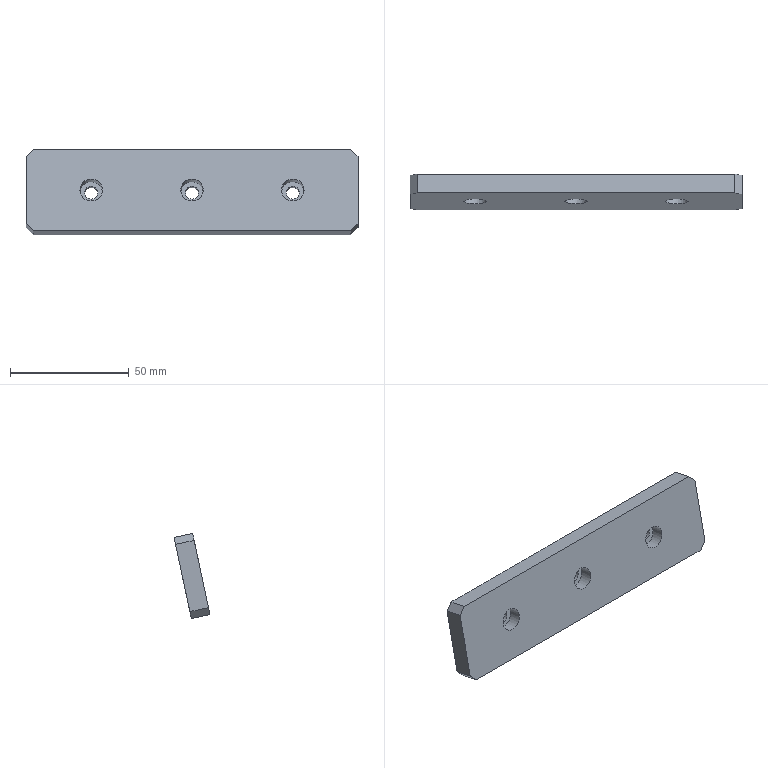Part | STEP file | P011002S004-005 | 1 solid | 19 faces | box 140 x 15.102 x 35.898 mm | volume 37708 mm3 | plane 13 | cylinder 6 | commonest cylinder face diameters 5.5 x3 9.5 x3
STEP:
#1=CARTESIAN_POINT('',(0.,0.,0.));
#2=DIRECTION('',(0.,0.,1.));
#3=DIRECTION('',(1.,0.,0.));
#4=AXIS2_PLACEMENT_3D('',#1,#2,#3);
#5=CARTESIAN_POINT('',(-47.25,-255.791,41.161));
#6=VERTEX_POINT('',#5);
#7=CARTESIAN_POINT('',(-42.5,-255.791,41.161));
#8=DIRECTION('',(0.,0.9781,-0.2079));
#9=DIRECTION('',(-1.,0.,0.));
#10=AXIS2_PLACEMENT_3D('',#7,#8,#9);
#11=CIRCLE('',#10,4.75);
#12=CARTESIAN_POINT('',(-5.,-253.192,53.388));
#13=DIRECTION('',(0.,-0.9781,0.2079));
#14=DIRECTION('',(0.,-0.2079,-0.9781));
#15=AXIS2_PLACEMENT_3D('',#12,#13,#14);
#16=PLANE('',#15);
#17=CARTESIAN_POINT('',(12.5,-42.25));
#18=CARTESIAN_POINT('',(4.273,-42.25));
#19=CARTESIAN_POINT('',(8.386,-35.125));
#20=CARTESIAN_POINT('',(12.5,-28.));
#21=CARTESIAN_POINT('',(16.614,-35.125));
#22=CARTESIAN_POINT('',(20.727,-42.25));
#23=CARTESIAN_POINT('',(12.5,-42.25));
#24=(BOUNDED_CURVE()B_SPLINE_CURVE(2,(#17,#18,#19,#20,#21,#22,#23),.UNSPECIFIED.,.T.,.F.)B_SPLINE_CURVE_WITH_KNOTS((1,2,2,2,2,1),(-2.094,0.,2.094,4.189,6.283,8.378),.UNSPECIFIED.)CURVE()GEOMETRIC_REPRESENTATION_ITEM()RATIONAL_B_SPLINE_CURVE((1.,0.5,1.,0.5,1.,0.5,1.))REPRESENTATION_ITEM(''));
#25=(GEOMETRIC_REPRESENTATION_CONTEXT(2)PARAMETRIC_REPRESENTATION_CONTEXT()REPRESENTATION_CONTEXT('',''));
#26=DEFINITIONAL_REPRESENTATION('',(#24),#25);
#27=PCURVE('',#16,#26);
#28=CARTESIAN_POINT('',(-42.5,-211.774,31.805));
#29=DIRECTION('',(0.,-0.9781,0.2079));
#30=DIRECTION('',(0.,-0.2079,-0.9781));
#31=AXIS2_PLACEMENT_3D('',#28,#29,#30);
#32=CYLINDRICAL_SURFACE('',#31,4.75);
#33=CARTESIAN_POINT('',(10.996,45.));
#34=DIRECTION('',(-1.,0.));
#35=VECTOR('',#34,1.);
#36=LINE('',#33,#35);
#37=(GEOMETRIC_REPRESENTATION_CONTEXT(2)PARAMETRIC_REPRESENTATION_CONTEXT()REPRESENTATION_CONTEXT('',''));
#38=DEFINITIONAL_REPRESENTATION('',(#36),#37);
#39=PCURVE('',#32,#38);
#40=SURFACE_CURVE('',#11,(#27,#39),.PCURVE_S1.);
#41=EDGE_CURVE('',#6,#6,#40,.T.);
#42=ORIENTED_EDGE('',*,*,#41,.T.);
#43=EDGE_LOOP('',(#42));
#44=FACE_BOUND('',#43,.T.);
#45=CARTESIAN_POINT('',(37.75,-255.791,41.161));
#46=VERTEX_POINT('',#45);
#47=CARTESIAN_POINT('',(42.5,-255.791,41.161));
#48=DIRECTION('',(0.,0.9781,-0.2079));
#49=DIRECTION('',(-1.,0.,0.));
#50=AXIS2_PLACEMENT_3D('',#47,#48,#49);
#51=CIRCLE('',#50,4.75);
#52=CARTESIAN_POINT('',(12.5,42.75));
#53=CARTESIAN_POINT('',(4.273,42.75));
#54=CARTESIAN_POINT('',(8.386,49.875));
#55=CARTESIAN_POINT('',(12.5,57.));
#56=CARTESIAN_POINT('',(16.614,49.875));
#57=CARTESIAN_POINT('',(20.727,42.75));
#58=CARTESIAN_POINT('',(12.5,42.75));
#59=(BOUNDED_CURVE()B_SPLINE_CURVE(2,(#52,#53,#54,#55,#56,#57,#58),.UNSPECIFIED.,.T.,.F.)B_SPLINE_CURVE_WITH_KNOTS((1,2,2,2,2,1),(-2.094,0.,2.094,4.189,6.283,8.378),.UNSPECIFIED.)CURVE()GEOMETRIC_REPRESENTATION_ITEM()RATIONAL_B_SPLINE_CURVE((1.,0.5,1.,0.5,1.,0.5,1.))REPRESENTATION_ITEM(''));
#60=(GEOMETRIC_REPRESENTATION_CONTEXT(2)PARAMETRIC_REPRESENTATION_CONTEXT()REPRESENTATION_CONTEXT('',''));
#61=DEFINITIONAL_REPRESENTATION('',(#59),#60);
#62=PCURVE('',#16,#61);
#63=CARTESIAN_POINT('',(42.5,-211.774,31.805));
#64=DIRECTION('',(0.,-0.9781,0.2079));
#65=DIRECTION('',(0.,-0.2079,-0.9781));
#66=AXIS2_PLACEMENT_3D('',#63,#64,#65);
#67=CYLINDRICAL_SURFACE('',#66,4.75);
#68=CARTESIAN_POINT('',(10.996,45.));
#69=DIRECTION('',(-1.,0.));
#70=VECTOR('',#69,1.);
#71=LINE('',#68,#70);
#72=(GEOMETRIC_REPRESENTATION_CONTEXT(2)PARAMETRIC_REPRESENTATION_CONTEXT()REPRESENTATION_CONTEXT('',''));
#73=DEFINITIONAL_REPRESENTATION('',(#71),#72);
#74=PCURVE('',#67,#73);
#75=SURFACE_CURVE('',#51,(#62,#74),.PCURVE_S1.);
#76=EDGE_CURVE('',#46,#46,#75,.T.);
#77=ORIENTED_EDGE('',*,*,#76,.T.);
#78=EDGE_LOOP('',(#77));
#79=FACE_BOUND('',#78,.T.);
#80=CARTESIAN_POINT('',(-4.75,-255.791,41.161));
#81=VERTEX_POINT('',#80);
#82=CARTESIAN_POINT('',(0.,-255.791,41.161));
#83=DIRECTION('',(0.,0.9781,-0.2079));
#84=DIRECTION('',(-1.,0.,0.));
#85=AXIS2_PLACEMENT_3D('',#82,#83,#84);
#86=CIRCLE('',#85,4.75);
#87=CARTESIAN_POINT('',(12.5,0.25));
#88=CARTESIAN_POINT('',(4.273,0.25));
#89=CARTESIAN_POINT('',(8.386,7.375));
#90=CARTESIAN_POINT('',(12.5,14.5));
#91=CARTESIAN_POINT('',(16.614,7.375));
#92=CARTESIAN_POINT('',(20.727,0.25));
#93=CARTESIAN_POINT('',(12.5,0.25));
#94=(BOUNDED_CURVE()B_SPLINE_CURVE(2,(#87,#88,#89,#90,#91,#92,#93),.UNSPECIFIED.,.T.,.F.)B_SPLINE_CURVE_WITH_KNOTS((1,2,2,2,2,1),(-2.094,0.,2.094,4.189,6.283,8.378),.UNSPECIFIED.)CURVE()GEOMETRIC_REPRESENTATION_ITEM()RATIONAL_B_SPLINE_CURVE((1.,0.5,1.,0.5,1.,0.5,1.))REPRESENTATION_ITEM(''));
#95=(GEOMETRIC_REPRESENTATION_CONTEXT(2)PARAMETRIC_REPRESENTATION_CONTEXT()REPRESENTATION_CONTEXT('',''));
#96=DEFINITIONAL_REPRESENTATION('',(#94),#95);
#97=PCURVE('',#16,#96);
#98=CARTESIAN_POINT('',(0.,-211.774,31.805));
#99=DIRECTION('',(0.,-0.9781,0.2079));
#100=DIRECTION('',(0.,-0.2079,-0.9781));
#101=AXIS2_PLACEMENT_3D('',#98,#99,#100);
#102=CYLINDRICAL_SURFACE('',#101,4.75);
#103=CARTESIAN_POINT('',(10.996,45.));
#104=DIRECTION('',(-1.,0.));
#105=VECTOR('',#104,1.);
#106=LINE('',#103,#105);
#107=(GEOMETRIC_REPRESENTATION_CONTEXT(2)PARAMETRIC_REPRESENTATION_CONTEXT()REPRESENTATION_CONTEXT('',''));
#108=DEFINITIONAL_REPRESENTATION('',(#106),#107);
#109=PCURVE('',#102,#108);
#110=SURFACE_CURVE('',#86,(#97,#109),.PCURVE_S1.);
#111=EDGE_CURVE('',#81,#81,#110,.T.);
#112=ORIENTED_EDGE('',*,*,#111,.T.);
#113=EDGE_LOOP('',(#112));
#114=FACE_BOUND('',#113,.T.);
#115=CARTESIAN_POINT('',(-67.,-259.429,24.044));
#116=VERTEX_POINT('',#115);
#117=CARTESIAN_POINT('',(67.,-259.429,24.044));
#118=VERTEX_POINT('',#117);
#119=CARTESIAN_POINT('',(-5.,-259.429,24.044));
#120=DIRECTION('',(1.,0.,0.));
#121=VECTOR('',#120,1.);
#122=LINE('',#119,#121);
#123=CARTESIAN_POINT('',(30.,0.));
#124=DIRECTION('',(0.,1.));
#125=VECTOR('',#124,1.);
#126=LINE('',#123,#125);
#127=(GEOMETRIC_REPRESENTATION_CONTEXT(2)PARAMETRIC_REPRESENTATION_CONTEXT()REPRESENTATION_CONTEXT('',''));
#128=DEFINITIONAL_REPRESENTATION('',(#126),#127);
#129=PCURVE('',#16,#128);
#130=CARTESIAN_POINT('',(-5.,-258.94,23.94));
#131=DIRECTION('',(0.,-0.2079,-0.9781));
#132=DIRECTION('',(0.,0.9781,-0.2079));
#133=AXIS2_PLACEMENT_3D('',#130,#131,#132);
#134=PLANE('',#133);
#135=CARTESIAN_POINT('',(-0.5,0.));
#136=DIRECTION('',(0.,1.));
#137=VECTOR('',#136,1.);
#138=LINE('',#135,#137);
#139=(GEOMETRIC_REPRESENTATION_CONTEXT(2)PARAMETRIC_REPRESENTATION_CONTEXT()REPRESENTATION_CONTEXT('',''));
#140=DEFINITIONAL_REPRESENTATION('',(#138),#139);
#141=PCURVE('',#134,#140);
#142=SURFACE_CURVE('',#122,(#129,#141),.PCURVE_S1.);
#143=EDGE_CURVE('',#116,#118,#142,.T.);
#144=ORIENTED_EDGE('',*,*,#143,.T.);
#145=CARTESIAN_POINT('',(70.,-258.806,26.978));
#146=VERTEX_POINT('',#145);
#147=CARTESIAN_POINT('',(46.,-263.795,3.503));
#148=DIRECTION('',(-0.7071,-0.147,-0.6917));
#149=VECTOR('',#148,1.);
#150=LINE('',#147,#149);
#151=CARTESIAN_POINT('',(51.,51.));
#152=DIRECTION('',(0.7071,-0.7071));
#153=VECTOR('',#152,1.);
#154=LINE('',#151,#153);
#155=(GEOMETRIC_REPRESENTATION_CONTEXT(2)PARAMETRIC_REPRESENTATION_CONTEXT()REPRESENTATION_CONTEXT('',''));
#156=DEFINITIONAL_REPRESENTATION('',(#154),#155);
#157=PCURVE('',#16,#156);
#158=CARTESIAN_POINT('',(70.,-186.887,11.691));
#159=DIRECTION('',(-0.7071,0.147,0.6917));
#160=DIRECTION('',(-0.6993,0.,-0.7149));
#161=AXIS2_PLACEMENT_3D('',#158,#159,#160);
#162=PLANE('',#161);
#163=CARTESIAN_POINT('',(22.636,77.753));
#164=DIRECTION('',(0.9889,0.1486));
#165=VECTOR('',#164,1.);
#166=LINE('',#163,#165);
#167=(GEOMETRIC_REPRESENTATION_CONTEXT(2)PARAMETRIC_REPRESENTATION_CONTEXT()REPRESENTATION_CONTEXT('',''));
#168=DEFINITIONAL_REPRESENTATION('',(#166),#167);
#169=PCURVE('',#162,#168);
#170=SURFACE_CURVE('',#150,(#157,#169),.PCURVE_S1.);
#171=EDGE_CURVE('',#146,#118,#170,.T.);
#172=ORIENTED_EDGE('',*,*,#171,.F.);
#173=CARTESIAN_POINT('',(70.,-252.776,55.344));
#174=VERTEX_POINT('',#173);
#175=CARTESIAN_POINT('',(70.,-271.918,-34.713));
#176=DIRECTION('',(0.,0.2079,0.9781));
#177=VECTOR('',#176,1.);
#178=LINE('',#175,#177);
#179=CARTESIAN_POINT('',(90.07,75.));
#180=DIRECTION('',(-1.,0.));
#181=VECTOR('',#180,1.);
#182=LINE('',#179,#181);
#183=(GEOMETRIC_REPRESENTATION_CONTEXT(2)PARAMETRIC_REPRESENTATION_CONTEXT()REPRESENTATION_CONTEXT('',''));
#184=DEFINITIONAL_REPRESENTATION('',(#182),#183);
#185=PCURVE('',#16,#184);
#186=CARTESIAN_POINT('',(70.,-200.,-50.));
#187=DIRECTION('',(1.,0.,0.));
#188=DIRECTION('',(0.,0.,1.));
#189=AXIS2_PLACEMENT_3D('',#186,#187,#188);
#190=PLANE('',#189);
#191=CARTESIAN_POINT('',(15.287,71.918));
#192=DIRECTION('',(0.9781,-0.2079));
#193=VECTOR('',#192,1.);
#194=LINE('',#191,#193);
#195=(GEOMETRIC_REPRESENTATION_CONTEXT(2)PARAMETRIC_REPRESENTATION_CONTEXT()REPRESENTATION_CONTEXT('',''));
#196=DEFINITIONAL_REPRESENTATION('',(#194),#195);
#197=PCURVE('',#190,#196);
#198=SURFACE_CURVE('',#178,(#185,#197),.PCURVE_S1.);
#199=EDGE_CURVE('',#146,#174,#198,.T.);
#200=ORIENTED_EDGE('',*,*,#199,.T.);
#201=CARTESIAN_POINT('',(67.,-252.152,58.279));
#202=VERTEX_POINT('',#201);
#203=CARTESIAN_POINT('',(33.5,-245.187,91.047));
#204=DIRECTION('',(0.7071,-0.147,-0.6917));
#205=VECTOR('',#204,1.);
#206=LINE('',#203,#205);
#207=CARTESIAN_POINT('',(-38.5,38.5));
#208=DIRECTION('',(0.7071,0.7071));
#209=VECTOR('',#208,1.);
#210=LINE('',#207,#209);
#211=(GEOMETRIC_REPRESENTATION_CONTEXT(2)PARAMETRIC_REPRESENTATION_CONTEXT()REPRESENTATION_CONTEXT('',''));
#212=DEFINITIONAL_REPRESENTATION('',(#210),#211);
#213=PCURVE('',#16,#212);
#214=CARTESIAN_POINT('',(67.,-251.663,58.175));
#215=DIRECTION('',(-0.7071,-0.147,-0.6917));
#216=DIRECTION('',(0.6993,0.,-0.7149));
#217=AXIS2_PLACEMENT_3D('',#214,#215,#216);
#218=PLANE('',#217);
#219=CARTESIAN_POINT('',(-46.924,-6.547));
#220=DIRECTION('',(0.9889,0.1486));
#221=VECTOR('',#220,1.);
#222=LINE('',#219,#221);
#223=(GEOMETRIC_REPRESENTATION_CONTEXT(2)PARAMETRIC_REPRESENTATION_CONTEXT()REPRESENTATION_CONTEXT('',''));
#224=DEFINITIONAL_REPRESENTATION('',(#222),#223);
#225=PCURVE('',#218,#224);
#226=SURFACE_CURVE('',#206,(#213,#225),.PCURVE_S1.);
#227=EDGE_CURVE('',#202,#174,#226,.T.);
#228=ORIENTED_EDGE('',*,*,#227,.F.);
#229=CARTESIAN_POINT('',(-67.,-252.152,58.279));
#230=VERTEX_POINT('',#229);
#231=CARTESIAN_POINT('',(-5.,-252.152,58.279));
#232=DIRECTION('',(-1.,0.,0.));
#233=VECTOR('',#232,1.);
#234=LINE('',#231,#233);
#235=CARTESIAN_POINT('',(-5.,0.));
#236=DIRECTION('',(0.,-1.));
#237=VECTOR('',#236,1.);
#238=LINE('',#235,#237);
#239=(GEOMETRIC_REPRESENTATION_CONTEXT(2)PARAMETRIC_REPRESENTATION_CONTEXT()REPRESENTATION_CONTEXT('',''));
#240=DEFINITIONAL_REPRESENTATION('',(#238),#239);
#241=PCURVE('',#16,#240);
#242=CARTESIAN_POINT('',(-5.,-251.663,58.175));
#243=DIRECTION('',(0.,0.2079,0.9781));
#244=DIRECTION('',(0.,-0.9781,0.2079));
#245=AXIS2_PLACEMENT_3D('',#242,#243,#244);
#246=PLANE('',#245);
#247=CARTESIAN_POINT('',(0.5,0.));
#248=DIRECTION('',(0.,-1.));
#249=VECTOR('',#248,1.);
#250=LINE('',#247,#249);
#251=(GEOMETRIC_REPRESENTATION_CONTEXT(2)PARAMETRIC_REPRESENTATION_CONTEXT()REPRESENTATION_CONTEXT('',''));
#252=DEFINITIONAL_REPRESENTATION('',(#250),#251);
#253=PCURVE('',#246,#252);
#254=SURFACE_CURVE('',#234,(#241,#253),.PCURVE_S1.);
#255=EDGE_CURVE('',#202,#230,#254,.T.);
#256=ORIENTED_EDGE('',*,*,#255,.T.);
#257=CARTESIAN_POINT('',(-70.,-252.776,55.344));
#258=VERTEX_POINT('',#257);
#259=CARTESIAN_POINT('',(-38.5,-246.227,86.156));
#260=DIRECTION('',(0.7071,0.147,0.6917));
#261=VECTOR('',#260,1.);
#262=LINE('',#259,#261);
#263=CARTESIAN_POINT('',(-33.5,-33.5));
#264=DIRECTION('',(-0.7071,0.7071));
#265=VECTOR('',#264,1.);
#266=LINE('',#263,#265);
#267=(GEOMETRIC_REPRESENTATION_CONTEXT(2)PARAMETRIC_REPRESENTATION_CONTEXT()REPRESENTATION_CONTEXT('',''));
#268=DEFINITIONAL_REPRESENTATION('',(#266),#267);
#269=PCURVE('',#16,#268);
#270=CARTESIAN_POINT('',(-70.,-180.858,40.058));
#271=DIRECTION('',(-0.7071,0.147,0.6917));
#272=DIRECTION('',(-0.6993,0.,-0.7149));
#273=AXIS2_PLACEMENT_3D('',#270,#271,#272);
#274=PLANE('',#273);
#275=CARTESIAN_POINT('',(-54.981,66.087));
#276=DIRECTION('',(-0.9889,-0.1486));
#277=VECTOR('',#276,1.);
#278=LINE('',#275,#277);
#279=(GEOMETRIC_REPRESENTATION_CONTEXT(2)PARAMETRIC_REPRESENTATION_CONTEXT()REPRESENTATION_CONTEXT('',''));
#280=DEFINITIONAL_REPRESENTATION('',(#278),#279);
#281=PCURVE('',#274,#280);
#282=SURFACE_CURVE('',#262,(#269,#281),.PCURVE_S1.);
#283=EDGE_CURVE('',#258,#230,#282,.T.);
#284=ORIENTED_EDGE('',*,*,#283,.F.);
#285=CARTESIAN_POINT('',(-70.,-258.806,26.978));
#286=VERTEX_POINT('',#285);
#287=CARTESIAN_POINT('',(-70.,-271.918,-34.713));
#288=DIRECTION('',(0.,-0.2079,-0.9781));
#289=VECTOR('',#288,1.);
#290=LINE('',#287,#289);
#291=CARTESIAN_POINT('',(90.07,-65.));
#292=DIRECTION('',(1.,0.));
#293=VECTOR('',#292,1.);
#294=LINE('',#291,#293);
#295=(GEOMETRIC_REPRESENTATION_CONTEXT(2)PARAMETRIC_REPRESENTATION_CONTEXT()REPRESENTATION_CONTEXT('',''));
#296=DEFINITIONAL_REPRESENTATION('',(#294),#295);
#297=PCURVE('',#16,#296);
#298=CARTESIAN_POINT('',(-70.,-200.,-50.));
#299=DIRECTION('',(1.,0.,0.));
#300=DIRECTION('',(0.,0.,1.));
#301=AXIS2_PLACEMENT_3D('',#298,#299,#300);
#302=PLANE('',#301);
#303=CARTESIAN_POINT('',(15.287,71.918));
#304=DIRECTION('',(-0.9781,0.2079));
#305=VECTOR('',#304,1.);
#306=LINE('',#303,#305);
#307=(GEOMETRIC_REPRESENTATION_CONTEXT(2)PARAMETRIC_REPRESENTATION_CONTEXT()REPRESENTATION_CONTEXT('',''));
#308=DEFINITIONAL_REPRESENTATION('',(#306),#307);
#309=PCURVE('',#302,#308);
#310=SURFACE_CURVE('',#290,(#297,#309),.PCURVE_S1.);
#311=EDGE_CURVE('',#258,#286,#310,.T.);
#312=ORIENTED_EDGE('',*,*,#311,.T.);
#313=CARTESIAN_POINT('',(-51.,-262.756,8.393));
#314=DIRECTION('',(-0.7071,0.147,0.6917));
#315=VECTOR('',#314,1.);
#316=LINE('',#313,#315);
#317=CARTESIAN_POINT('',(46.,-46.));
#318=DIRECTION('',(-0.7071,-0.7071));
#319=VECTOR('',#318,1.);
#320=LINE('',#317,#319);
#321=(GEOMETRIC_REPRESENTATION_CONTEXT(2)PARAMETRIC_REPRESENTATION_CONTEXT()REPRESENTATION_CONTEXT('',''));
#322=DEFINITIONAL_REPRESENTATION('',(#320),#321);
#323=PCURVE('',#16,#322);
#324=CARTESIAN_POINT('',(-67.,-258.94,23.94));
#325=DIRECTION('',(-0.7071,-0.147,-0.6917));
#326=DIRECTION('',(0.6993,0.,-0.7149));
#327=AXIS2_PLACEMENT_3D('',#324,#325,#326);
#328=PLANE('',#327);
#329=CARTESIAN_POINT('',(22.302,3.858));
#330=DIRECTION('',(-0.9889,-0.1486));
#331=VECTOR('',#330,1.);
#332=LINE('',#329,#331);
#333=(GEOMETRIC_REPRESENTATION_CONTEXT(2)PARAMETRIC_REPRESENTATION_CONTEXT()REPRESENTATION_CONTEXT('',''));
#334=DEFINITIONAL_REPRESENTATION('',(#332),#333);
#335=PCURVE('',#328,#334);
#336=SURFACE_CURVE('',#316,(#323,#335),.PCURVE_S1.);
#337=EDGE_CURVE('',#116,#286,#336,.T.);
#338=ORIENTED_EDGE('',*,*,#337,.F.);
#339=EDGE_LOOP('',(#144,#172,#200,#228,#256,#284,#312,#338));
#340=FACE_BOUND('',#339,.T.);
#341=ADVANCED_FACE('',(#44,#79,#114,#340),#16,.T.);
#342=CARTESIAN_POINT('',(70.,-244.951,53.681));
#343=VERTEX_POINT('',#342);
#344=CARTESIAN_POINT('',(70.,-250.98,25.315));
#345=VERTEX_POINT('',#344);
#346=CARTESIAN_POINT('',(70.,-264.093,-36.377));
#347=DIRECTION('',(0.,-0.2079,-0.9781));
#348=VECTOR('',#347,1.);
#349=LINE('',#346,#348);
#350=CARTESIAN_POINT('',(13.623,64.093));
#351=DIRECTION('',(-0.9781,0.2079));
#352=VECTOR('',#351,1.);
#353=LINE('',#350,#352);
#354=(GEOMETRIC_REPRESENTATION_CONTEXT(2)PARAMETRIC_REPRESENTATION_CONTEXT()REPRESENTATION_CONTEXT('',''));
#355=DEFINITIONAL_REPRESENTATION('',(#353),#354);
#356=PCURVE('',#190,#355);
#357=CARTESIAN_POINT('',(-5.,-245.367,51.725));
#358=DIRECTION('',(0.,0.9781,-0.2079));
#359=DIRECTION('',(0.,0.2079,0.9781));
#360=AXIS2_PLACEMENT_3D('',#357,#358,#359);
#361=PLANE('',#360);
#362=CARTESIAN_POINT('',(-90.07,75.));
#363=DIRECTION('',(-1.,0.));
#364=VECTOR('',#363,1.);
#365=LINE('',#362,#364);
#366=(GEOMETRIC_REPRESENTATION_CONTEXT(2)PARAMETRIC_REPRESENTATION_CONTEXT()REPRESENTATION_CONTEXT('',''));
#367=DEFINITIONAL_REPRESENTATION('',(#365),#366);
#368=PCURVE('',#361,#367);
#369=SURFACE_CURVE('',#349,(#356,#368),.PCURVE_S1.);
#370=EDGE_CURVE('',#343,#345,#369,.T.);
#371=ORIENTED_EDGE('',*,*,#370,.F.);
#372=CARTESIAN_POINT('',(70.,-180.858,40.058));
#373=DIRECTION('',(0.,0.9781,-0.2079));
#374=VECTOR('',#373,1.);
#375=LINE('',#372,#374);
#376=CARTESIAN_POINT('',(90.058,-19.142));
#377=DIRECTION('',(-0.2079,-0.9781));
#378=VECTOR('',#377,1.);
#379=LINE('',#376,#378);
#380=(GEOMETRIC_REPRESENTATION_CONTEXT(2)PARAMETRIC_REPRESENTATION_CONTEXT()REPRESENTATION_CONTEXT('',''));
#381=DEFINITIONAL_REPRESENTATION('',(#379),#380);
#382=PCURVE('',#190,#381);
#383=CARTESIAN_POINT('',(15.049,-71.583));
#384=DIRECTION('',(0.1486,-0.9889));
#385=VECTOR('',#384,1.);
#386=LINE('',#383,#385);
#387=(GEOMETRIC_REPRESENTATION_CONTEXT(2)PARAMETRIC_REPRESENTATION_CONTEXT()REPRESENTATION_CONTEXT('',''));
#388=DEFINITIONAL_REPRESENTATION('',(#386),#387);
#389=PCURVE('',#218,#388);
#390=SURFACE_CURVE('',#375,(#382,#389),.PCURVE_S1.);
#391=EDGE_CURVE('',#174,#343,#390,.T.);
#392=ORIENTED_EDGE('',*,*,#391,.F.);
#393=ORIENTED_EDGE('',*,*,#199,.F.);
#394=CARTESIAN_POINT('',(70.,-186.887,11.691));
#395=DIRECTION('',(0.,-0.9781,0.2079));
#396=VECTOR('',#395,1.);
#397=LINE('',#394,#396);
#398=CARTESIAN_POINT('',(61.691,-13.113));
#399=DIRECTION('',(0.2079,0.9781));
#400=VECTOR('',#399,1.);
#401=LINE('',#398,#400);
#402=(GEOMETRIC_REPRESENTATION_CONTEXT(2)PARAMETRIC_REPRESENTATION_CONTEXT()REPRESENTATION_CONTEXT('',''));
#403=DEFINITIONAL_REPRESENTATION('',(#401),#402);
#404=PCURVE('',#190,#403);
#405=CARTESIAN_POINT('',(0.,0.));
#406=DIRECTION('',(-0.1486,0.9889));
#407=VECTOR('',#406,1.);
#408=LINE('',#405,#407);
#409=(GEOMETRIC_REPRESENTATION_CONTEXT(2)PARAMETRIC_REPRESENTATION_CONTEXT()REPRESENTATION_CONTEXT('',''));
#410=DEFINITIONAL_REPRESENTATION('',(#408),#409);
#411=PCURVE('',#162,#410);
#412=SURFACE_CURVE('',#397,(#404,#411),.PCURVE_S1.);
#413=EDGE_CURVE('',#345,#146,#412,.T.);
#414=ORIENTED_EDGE('',*,*,#413,.F.);
#415=EDGE_LOOP('',(#371,#392,#393,#414));
#416=FACE_BOUND('',#415,.T.);
#417=ADVANCED_FACE('',(#416),#190,.T.);
#418=ORIENTED_EDGE('',*,*,#255,.F.);
#419=CARTESIAN_POINT('',(67.,-244.327,56.615));
#420=VERTEX_POINT('',#419);
#421=CARTESIAN_POINT('',(67.,-251.663,58.175));
#422=DIRECTION('',(0.,-0.9781,0.2079));
#423=VECTOR('',#422,1.);
#424=LINE('',#421,#423);
#425=CARTESIAN_POINT('',(0.,72.));
#426=DIRECTION('',(1.,0.));
#427=VECTOR('',#426,1.);
#428=LINE('',#425,#427);
#429=(GEOMETRIC_REPRESENTATION_CONTEXT(2)PARAMETRIC_REPRESENTATION_CONTEXT()REPRESENTATION_CONTEXT('',''));
#430=DEFINITIONAL_REPRESENTATION('',(#428),#429);
#431=PCURVE('',#246,#430);
#432=CARTESIAN_POINT('',(0.,0.));
#433=DIRECTION('',(-0.1486,0.9889));
#434=VECTOR('',#433,1.);
#435=LINE('',#432,#434);
#436=(GEOMETRIC_REPRESENTATION_CONTEXT(2)PARAMETRIC_REPRESENTATION_CONTEXT()REPRESENTATION_CONTEXT('',''));
#437=DEFINITIONAL_REPRESENTATION('',(#435),#436);
#438=PCURVE('',#218,#437);
#439=SURFACE_CURVE('',#424,(#431,#438),.PCURVE_S1.);
#440=EDGE_CURVE('',#420,#202,#439,.T.);
#441=ORIENTED_EDGE('',*,*,#440,.F.);
#442=CARTESIAN_POINT('',(-67.,-244.327,56.615));
#443=VERTEX_POINT('',#442);
#444=CARTESIAN_POINT('',(-5.,-244.327,56.615));
#445=DIRECTION('',(1.,0.,0.));
#446=VECTOR('',#445,1.);
#447=LINE('',#444,#446);
#448=CARTESIAN_POINT('',(-7.5,0.));
#449=DIRECTION('',(0.,1.));
#450=VECTOR('',#449,1.);
#451=LINE('',#448,#450);
#452=(GEOMETRIC_REPRESENTATION_CONTEXT(2)PARAMETRIC_REPRESENTATION_CONTEXT()REPRESENTATION_CONTEXT('',''));
#453=DEFINITIONAL_REPRESENTATION('',(#451),#452);
#454=PCURVE('',#246,#453);
#455=CARTESIAN_POINT('',(5.,0.));
#456=DIRECTION('',(0.,1.));
#457=VECTOR('',#456,1.);
#458=LINE('',#455,#457);
#459=(GEOMETRIC_REPRESENTATION_CONTEXT(2)PARAMETRIC_REPRESENTATION_CONTEXT()REPRESENTATION_CONTEXT('',''));
#460=DEFINITIONAL_REPRESENTATION('',(#458),#459);
#461=PCURVE('',#361,#460);
#462=SURFACE_CURVE('',#447,(#454,#461),.PCURVE_S1.);
#463=EDGE_CURVE('',#443,#420,#462,.T.);
#464=ORIENTED_EDGE('',*,*,#463,.F.);
#465=CARTESIAN_POINT('',(-67.,-251.663,58.175));
#466=DIRECTION('',(0.,0.9781,-0.2079));
#467=VECTOR('',#466,1.);
#468=LINE('',#465,#467);
#469=CARTESIAN_POINT('',(0.,-62.));
#470=DIRECTION('',(-1.,0.));
#471=VECTOR('',#470,1.);
#472=LINE('',#469,#471);
#473=(GEOMETRIC_REPRESENTATION_CONTEXT(2)PARAMETRIC_REPRESENTATION_CONTEXT()REPRESENTATION_CONTEXT('',''));
#474=DEFINITIONAL_REPRESENTATION('',(#472),#473);
#475=PCURVE('',#246,#474);
#476=CARTESIAN_POINT('',(-15.049,71.583));
#477=DIRECTION('',(0.1486,-0.9889));
#478=VECTOR('',#477,1.);
#479=LINE('',#476,#478);
#480=(GEOMETRIC_REPRESENTATION_CONTEXT(2)PARAMETRIC_REPRESENTATION_CONTEXT()REPRESENTATION_CONTEXT('',''));
#481=DEFINITIONAL_REPRESENTATION('',(#479),#480);
#482=PCURVE('',#274,#481);
#483=SURFACE_CURVE('',#468,(#475,#482),.PCURVE_S1.);
#484=EDGE_CURVE('',#230,#443,#483,.T.);
#485=ORIENTED_EDGE('',*,*,#484,.F.);
#486=EDGE_LOOP('',(#418,#441,#464,#485));
#487=FACE_BOUND('',#486,.T.);
#488=ADVANCED_FACE('',(#487),#246,.T.);
#489=ORIENTED_EDGE('',*,*,#311,.F.);
#490=CARTESIAN_POINT('',(-70.,-244.951,53.681));
#491=VERTEX_POINT('',#490);
#492=CARTESIAN_POINT('',(-70.,-180.858,40.058));
#493=DIRECTION('',(0.,-0.9781,0.2079));
#494=VECTOR('',#493,1.);
#495=LINE('',#492,#494);
#496=CARTESIAN_POINT('',(90.058,-19.142));
#497=DIRECTION('',(0.2079,0.9781));
#498=VECTOR('',#497,1.);
#499=LINE('',#496,#498);
#500=(GEOMETRIC_REPRESENTATION_CONTEXT(2)PARAMETRIC_REPRESENTATION_CONTEXT()REPRESENTATION_CONTEXT('',''));
#501=DEFINITIONAL_REPRESENTATION('',(#499),#500);
#502=PCURVE('',#302,#501);
#503=CARTESIAN_POINT('',(0.,0.));
#504=DIRECTION('',(-0.1486,0.9889));
#505=VECTOR('',#504,1.);
#506=LINE('',#503,#505);
#507=(GEOMETRIC_REPRESENTATION_CONTEXT(2)PARAMETRIC_REPRESENTATION_CONTEXT()REPRESENTATION_CONTEXT('',''));
#508=DEFINITIONAL_REPRESENTATION('',(#506),#507);
#509=PCURVE('',#274,#508);
#510=SURFACE_CURVE('',#495,(#502,#509),.PCURVE_S1.);
#511=EDGE_CURVE('',#491,#258,#510,.T.);
#512=ORIENTED_EDGE('',*,*,#511,.F.);
#513=CARTESIAN_POINT('',(-70.,-250.98,25.315));
#514=VERTEX_POINT('',#513);
#515=CARTESIAN_POINT('',(-70.,-264.093,-36.377));
#516=DIRECTION('',(0.,0.2079,0.9781));
#517=VECTOR('',#516,1.);
#518=LINE('',#515,#517);
#519=CARTESIAN_POINT('',(13.623,64.093));
#520=DIRECTION('',(0.9781,-0.2079));
#521=VECTOR('',#520,1.);
#522=LINE('',#519,#521);
#523=(GEOMETRIC_REPRESENTATION_CONTEXT(2)PARAMETRIC_REPRESENTATION_CONTEXT()REPRESENTATION_CONTEXT('',''));
#524=DEFINITIONAL_REPRESENTATION('',(#522),#523);
#525=PCURVE('',#302,#524);
#526=CARTESIAN_POINT('',(-90.07,-65.));
#527=DIRECTION('',(1.,0.));
#528=VECTOR('',#527,1.);
#529=LINE('',#526,#528);
#530=(GEOMETRIC_REPRESENTATION_CONTEXT(2)PARAMETRIC_REPRESENTATION_CONTEXT()REPRESENTATION_CONTEXT('',''));
#531=DEFINITIONAL_REPRESENTATION('',(#529),#530);
#532=PCURVE('',#361,#531);
#533=SURFACE_CURVE('',#518,(#525,#532),.PCURVE_S1.);
#534=EDGE_CURVE('',#514,#491,#533,.T.);
#535=ORIENTED_EDGE('',*,*,#534,.F.);
#536=CARTESIAN_POINT('',(-70.,-186.887,11.691));
#537=DIRECTION('',(0.,0.9781,-0.2079));
#538=VECTOR('',#537,1.);
#539=LINE('',#536,#538);
#540=CARTESIAN_POINT('',(61.691,-13.113));
#541=DIRECTION('',(-0.2079,-0.9781));
#542=VECTOR('',#541,1.);
#543=LINE('',#540,#542);
#544=(GEOMETRIC_REPRESENTATION_CONTEXT(2)PARAMETRIC_REPRESENTATION_CONTEXT()REPRESENTATION_CONTEXT('',''));
#545=DEFINITIONAL_REPRESENTATION('',(#543),#544);
#546=PCURVE('',#302,#545);
#547=CARTESIAN_POINT('',(6.658,-72.845));
#548=DIRECTION('',(0.1486,-0.9889));
#549=VECTOR('',#548,1.);
#550=LINE('',#547,#549);
#551=(GEOMETRIC_REPRESENTATION_CONTEXT(2)PARAMETRIC_REPRESENTATION_CONTEXT()REPRESENTATION_CONTEXT('',''));
#552=DEFINITIONAL_REPRESENTATION('',(#550),#551);
#553=PCURVE('',#328,#552);
#554=SURFACE_CURVE('',#539,(#546,#553),.PCURVE_S1.);
#555=EDGE_CURVE('',#286,#514,#554,.T.);
#556=ORIENTED_EDGE('',*,*,#555,.F.);
#557=EDGE_LOOP('',(#489,#512,#535,#556));
#558=FACE_BOUND('',#557,.T.);
#559=ADVANCED_FACE('',(#558),#302,.F.);
#560=CARTESIAN_POINT('',(-42.5,-247.394,42.188));
#561=VERTEX_POINT('',#560);
#562=CARTESIAN_POINT('',(-42.5,-247.966,39.498));
#563=DIRECTION('',(0.,-0.9781,0.2079));
#564=DIRECTION('',(0.,0.2079,0.9781));
#565=AXIS2_PLACEMENT_3D('',#562,#563,#564);
#566=CIRCLE('',#565,2.75);
#567=CARTESIAN_POINT('',(-9.75,-37.5));
#568=CARTESIAN_POINT('',(-9.75,-42.263));
#569=CARTESIAN_POINT('',(-13.875,-39.882));
#570=CARTESIAN_POINT('',(-18.,-37.5));
#571=CARTESIAN_POINT('',(-13.875,-35.118));
#572=CARTESIAN_POINT('',(-9.75,-32.737));
#573=CARTESIAN_POINT('',(-9.75,-37.5));
#574=(BOUNDED_CURVE()B_SPLINE_CURVE(2,(#567,#568,#569,#570,#571,#572,#573),.UNSPECIFIED.,.T.,.F.)B_SPLINE_CURVE_WITH_KNOTS((1,2,2,2,2,1),(-2.094,0.,2.094,4.189,6.283,8.378),.UNSPECIFIED.)CURVE()GEOMETRIC_REPRESENTATION_ITEM()RATIONAL_B_SPLINE_CURVE((1.,0.5,1.,0.5,1.,0.5,1.))REPRESENTATION_ITEM(''));
#575=(GEOMETRIC_REPRESENTATION_CONTEXT(2)PARAMETRIC_REPRESENTATION_CONTEXT()REPRESENTATION_CONTEXT('',''));
#576=DEFINITIONAL_REPRESENTATION('',(#574),#575);
#577=PCURVE('',#361,#576);
#578=CARTESIAN_POINT('',(-42.5,-211.774,31.805));
#579=DIRECTION('',(0.,-0.9781,0.2079));
#580=DIRECTION('',(0.,-0.2079,-0.9781));
#581=AXIS2_PLACEMENT_3D('',#578,#579,#580);
#582=CYLINDRICAL_SURFACE('',#581,2.75);
#583=CARTESIAN_POINT('',(3.142,37.));
#584=DIRECTION('',(1.,0.));
#585=VECTOR('',#584,1.);
#586=LINE('',#583,#585);
#587=(GEOMETRIC_REPRESENTATION_CONTEXT(2)PARAMETRIC_REPRESENTATION_CONTEXT()REPRESENTATION_CONTEXT('',''));
#588=DEFINITIONAL_REPRESENTATION('',(#586),#587);
#589=PCURVE('',#582,#588);
#590=SURFACE_CURVE('',#566,(#577,#589),.PCURVE_S1.);
#591=EDGE_CURVE('',#561,#561,#590,.T.);
#592=ORIENTED_EDGE('',*,*,#591,.T.);
#593=EDGE_LOOP('',(#592));
#594=FACE_BOUND('',#593,.T.);
#595=CARTESIAN_POINT('',(42.5,-247.394,42.188));
#596=VERTEX_POINT('',#595);
#597=CARTESIAN_POINT('',(42.5,-247.966,39.498));
#598=DIRECTION('',(0.,-0.9781,0.2079));
#599=DIRECTION('',(0.,0.2079,0.9781));
#600=AXIS2_PLACEMENT_3D('',#597,#598,#599);
#601=CIRCLE('',#600,2.75);
#602=CARTESIAN_POINT('',(-9.75,47.5));
#603=CARTESIAN_POINT('',(-9.75,42.737));
#604=CARTESIAN_POINT('',(-13.875,45.118));
#605=CARTESIAN_POINT('',(-18.,47.5));
#606=CARTESIAN_POINT('',(-13.875,49.882));
#607=CARTESIAN_POINT('',(-9.75,52.263));
#608=CARTESIAN_POINT('',(-9.75,47.5));
#609=(BOUNDED_CURVE()B_SPLINE_CURVE(2,(#602,#603,#604,#605,#606,#607,#608),.UNSPECIFIED.,.T.,.F.)B_SPLINE_CURVE_WITH_KNOTS((1,2,2,2,2,1),(-2.094,0.,2.094,4.189,6.283,8.378),.UNSPECIFIED.)CURVE()GEOMETRIC_REPRESENTATION_ITEM()RATIONAL_B_SPLINE_CURVE((1.,0.5,1.,0.5,1.,0.5,1.))REPRESENTATION_ITEM(''));
#610=(GEOMETRIC_REPRESENTATION_CONTEXT(2)PARAMETRIC_REPRESENTATION_CONTEXT()REPRESENTATION_CONTEXT('',''));
#611=DEFINITIONAL_REPRESENTATION('',(#609),#610);
#612=PCURVE('',#361,#611);
#613=CARTESIAN_POINT('',(42.5,-211.774,31.805));
#614=DIRECTION('',(0.,-0.9781,0.2079));
#615=DIRECTION('',(0.,-0.2079,-0.9781));
#616=AXIS2_PLACEMENT_3D('',#613,#614,#615);
#617=CYLINDRICAL_SURFACE('',#616,2.75);
#618=CARTESIAN_POINT('',(3.142,37.));
#619=DIRECTION('',(1.,0.));
#620=VECTOR('',#619,1.);
#621=LINE('',#618,#620);
#622=(GEOMETRIC_REPRESENTATION_CONTEXT(2)PARAMETRIC_REPRESENTATION_CONTEXT()REPRESENTATION_CONTEXT('',''));
#623=DEFINITIONAL_REPRESENTATION('',(#621),#622);
#624=PCURVE('',#617,#623);
#625=SURFACE_CURVE('',#601,(#612,#624),.PCURVE_S1.);
#626=EDGE_CURVE('',#596,#596,#625,.T.);
#627=ORIENTED_EDGE('',*,*,#626,.T.);
#628=EDGE_LOOP('',(#627));
#629=FACE_BOUND('',#628,.T.);
#630=CARTESIAN_POINT('',(0.,-247.394,42.188));
#631=VERTEX_POINT('',#630);
#632=CARTESIAN_POINT('',(0.,-247.966,39.498));
#633=DIRECTION('',(0.,-0.9781,0.2079));
#634=DIRECTION('',(0.,0.2079,0.9781));
#635=AXIS2_PLACEMENT_3D('',#632,#633,#634);
#636=CIRCLE('',#635,2.75);
#637=CARTESIAN_POINT('',(-9.75,5.));
#638=CARTESIAN_POINT('',(-9.75,0.2369));
#639=CARTESIAN_POINT('',(-13.875,2.618));
#640=CARTESIAN_POINT('',(-18.,5.));
#641=CARTESIAN_POINT('',(-13.875,7.382));
#642=CARTESIAN_POINT('',(-9.75,9.763));
#643=CARTESIAN_POINT('',(-9.75,5.));
#644=(BOUNDED_CURVE()B_SPLINE_CURVE(2,(#637,#638,#639,#640,#641,#642,#643),.UNSPECIFIED.,.T.,.F.)B_SPLINE_CURVE_WITH_KNOTS((1,2,2,2,2,1),(-2.094,0.,2.094,4.189,6.283,8.378),.UNSPECIFIED.)CURVE()GEOMETRIC_REPRESENTATION_ITEM()RATIONAL_B_SPLINE_CURVE((1.,0.5,1.,0.5,1.,0.5,1.))REPRESENTATION_ITEM(''));
#645=(GEOMETRIC_REPRESENTATION_CONTEXT(2)PARAMETRIC_REPRESENTATION_CONTEXT()REPRESENTATION_CONTEXT('',''));
#646=DEFINITIONAL_REPRESENTATION('',(#644),#645);
#647=PCURVE('',#361,#646);
#648=CARTESIAN_POINT('',(0.,-211.774,31.805));
#649=DIRECTION('',(0.,-0.9781,0.2079));
#650=DIRECTION('',(0.,-0.2079,-0.9781));
#651=AXIS2_PLACEMENT_3D('',#648,#649,#650);
#652=CYLINDRICAL_SURFACE('',#651,2.75);
#653=CARTESIAN_POINT('',(3.142,37.));
#654=DIRECTION('',(1.,0.));
#655=VECTOR('',#654,1.);
#656=LINE('',#653,#655);
#657=(GEOMETRIC_REPRESENTATION_CONTEXT(2)PARAMETRIC_REPRESENTATION_CONTEXT()REPRESENTATION_CONTEXT('',''));
#658=DEFINITIONAL_REPRESENTATION('',(#656),#657);
#659=PCURVE('',#652,#658);
#660=SURFACE_CURVE('',#636,(#647,#659),.PCURVE_S1.);
#661=EDGE_CURVE('',#631,#631,#660,.T.);
#662=ORIENTED_EDGE('',*,*,#661,.T.);
#663=EDGE_LOOP('',(#662));
#664=FACE_BOUND('',#663,.T.);
#665=ORIENTED_EDGE('',*,*,#534,.T.);
#666=CARTESIAN_POINT('',(-38.5,-238.402,84.493));
#667=DIRECTION('',(-0.7071,-0.147,-0.6917));
#668=VECTOR('',#667,1.);
#669=LINE('',#666,#668);
#670=CARTESIAN_POINT('',(33.5,-33.5));
#671=DIRECTION('',(-0.7071,-0.7071));
#672=VECTOR('',#671,1.);
#673=LINE('',#670,#672);
#674=(GEOMETRIC_REPRESENTATION_CONTEXT(2)PARAMETRIC_REPRESENTATION_CONTEXT()REPRESENTATION_CONTEXT('',''));
#675=DEFINITIONAL_REPRESENTATION('',(#673),#674);
#676=PCURVE('',#361,#675);
#677=CARTESIAN_POINT('',(-53.792,58.176));
#678=DIRECTION('',(0.9889,0.1486));
#679=VECTOR('',#678,1.);
#680=LINE('',#677,#679);
#681=(GEOMETRIC_REPRESENTATION_CONTEXT(2)PARAMETRIC_REPRESENTATION_CONTEXT()REPRESENTATION_CONTEXT('',''));
#682=DEFINITIONAL_REPRESENTATION('',(#680),#681);
#683=PCURVE('',#274,#682);
#684=SURFACE_CURVE('',#669,(#676,#683),.PCURVE_S1.);
#685=EDGE_CURVE('',#443,#491,#684,.T.);
#686=ORIENTED_EDGE('',*,*,#685,.F.);
#687=ORIENTED_EDGE('',*,*,#463,.T.);
#688=CARTESIAN_POINT('',(33.5,-237.362,89.383));
#689=DIRECTION('',(-0.7071,0.147,0.6917));
#690=VECTOR('',#689,1.);
#691=LINE('',#688,#690);
#692=CARTESIAN_POINT('',(38.5,38.5));
#693=DIRECTION('',(0.7071,-0.7071));
#694=VECTOR('',#693,1.);
#695=LINE('',#692,#694);
#696=(GEOMETRIC_REPRESENTATION_CONTEXT(2)PARAMETRIC_REPRESENTATION_CONTEXT()REPRESENTATION_CONTEXT('',''));
#697=DEFINITIONAL_REPRESENTATION('',(#695),#696);
#698=PCURVE('',#361,#697);
#699=CARTESIAN_POINT('',(-45.735,-14.458));
#700=DIRECTION('',(-0.9889,-0.1486));
#701=VECTOR('',#700,1.);
#702=LINE('',#699,#701);
#703=(GEOMETRIC_REPRESENTATION_CONTEXT(2)PARAMETRIC_REPRESENTATION_CONTEXT()REPRESENTATION_CONTEXT('',''));
#704=DEFINITIONAL_REPRESENTATION('',(#702),#703);
#705=PCURVE('',#218,#704);
#706=SURFACE_CURVE('',#691,(#698,#705),.PCURVE_S1.);
#707=EDGE_CURVE('',#343,#420,#706,.T.);
#708=ORIENTED_EDGE('',*,*,#707,.F.);
#709=ORIENTED_EDGE('',*,*,#370,.T.);
#710=CARTESIAN_POINT('',(67.,-251.604,22.38));
#711=VERTEX_POINT('',#710);
#712=CARTESIAN_POINT('',(46.,-255.97,1.839));
#713=DIRECTION('',(0.7071,0.147,0.6917));
#714=VECTOR('',#713,1.);
#715=LINE('',#712,#714);
#716=CARTESIAN_POINT('',(-51.,51.));
#717=DIRECTION('',(0.7071,0.7071));
#718=VECTOR('',#717,1.);
#719=LINE('',#716,#718);
#720=(GEOMETRIC_REPRESENTATION_CONTEXT(2)PARAMETRIC_REPRESENTATION_CONTEXT()REPRESENTATION_CONTEXT('',''));
#721=DEFINITIONAL_REPRESENTATION('',(#719),#720);
#722=PCURVE('',#361,#721);
#723=CARTESIAN_POINT('',(23.825,69.842));
#724=DIRECTION('',(-0.9889,-0.1486));
#725=VECTOR('',#724,1.);
#726=LINE('',#723,#725);
#727=(GEOMETRIC_REPRESENTATION_CONTEXT(2)PARAMETRIC_REPRESENTATION_CONTEXT()REPRESENTATION_CONTEXT('',''));
#728=DEFINITIONAL_REPRESENTATION('',(#726),#727);
#729=PCURVE('',#162,#728);
#730=SURFACE_CURVE('',#715,(#722,#729),.PCURVE_S1.);
#731=EDGE_CURVE('',#711,#345,#730,.T.);
#732=ORIENTED_EDGE('',*,*,#731,.F.);
#733=CARTESIAN_POINT('',(-67.,-251.604,22.38));
#734=VERTEX_POINT('',#733);
#735=CARTESIAN_POINT('',(-5.,-251.604,22.38));
#736=DIRECTION('',(-1.,0.,0.));
#737=VECTOR('',#736,1.);
#738=LINE('',#735,#737);
#739=CARTESIAN_POINT('',(-30.,0.));
#740=DIRECTION('',(0.,-1.));
#741=VECTOR('',#740,1.);
#742=LINE('',#739,#741);
#743=(GEOMETRIC_REPRESENTATION_CONTEXT(2)PARAMETRIC_REPRESENTATION_CONTEXT()REPRESENTATION_CONTEXT('',''));
#744=DEFINITIONAL_REPRESENTATION('',(#742),#743);
#745=PCURVE('',#361,#744);
#746=CARTESIAN_POINT('',(7.5,0.));
#747=DIRECTION('',(0.,-1.));
#748=VECTOR('',#747,1.);
#749=LINE('',#746,#748);
#750=(GEOMETRIC_REPRESENTATION_CONTEXT(2)PARAMETRIC_REPRESENTATION_CONTEXT()REPRESENTATION_CONTEXT('',''));
#751=DEFINITIONAL_REPRESENTATION('',(#749),#750);
#752=PCURVE('',#134,#751);
#753=SURFACE_CURVE('',#738,(#745,#752),.PCURVE_S1.);
#754=EDGE_CURVE('',#711,#734,#753,.T.);
#755=ORIENTED_EDGE('',*,*,#754,.T.);
#756=CARTESIAN_POINT('',(-51.,-254.931,6.73));
#757=DIRECTION('',(0.7071,-0.147,-0.6917));
#758=VECTOR('',#757,1.);
#759=LINE('',#756,#758);
#760=CARTESIAN_POINT('',(-46.,-46.));
#761=DIRECTION('',(-0.7071,0.7071));
#762=VECTOR('',#761,1.);
#763=LINE('',#760,#762);
#764=(GEOMETRIC_REPRESENTATION_CONTEXT(2)PARAMETRIC_REPRESENTATION_CONTEXT()REPRESENTATION_CONTEXT('',''));
#765=DEFINITIONAL_REPRESENTATION('',(#763),#764);
#766=PCURVE('',#361,#765);
#767=CARTESIAN_POINT('',(23.491,-4.054));
#768=DIRECTION('',(0.9889,0.1486));
#769=VECTOR('',#768,1.);
#770=LINE('',#767,#769);
#771=(GEOMETRIC_REPRESENTATION_CONTEXT(2)PARAMETRIC_REPRESENTATION_CONTEXT()REPRESENTATION_CONTEXT('',''));
#772=DEFINITIONAL_REPRESENTATION('',(#770),#771);
#773=PCURVE('',#328,#772);
#774=SURFACE_CURVE('',#759,(#766,#773),.PCURVE_S1.);
#775=EDGE_CURVE('',#514,#734,#774,.T.);
#776=ORIENTED_EDGE('',*,*,#775,.F.);
#777=EDGE_LOOP('',(#665,#686,#687,#708,#709,#732,#755,#776));
#778=FACE_BOUND('',#777,.T.);
#779=ADVANCED_FACE('',(#594,#629,#664,#778),#361,.T.);
#780=ORIENTED_EDGE('',*,*,#754,.F.);
#781=CARTESIAN_POINT('',(67.,-258.94,23.94));
#782=DIRECTION('',(0.,0.9781,-0.2079));
#783=VECTOR('',#782,1.);
#784=LINE('',#781,#783);
#785=CARTESIAN_POINT('',(0.,72.));
#786=DIRECTION('',(1.,0.));
#787=VECTOR('',#786,1.);
#788=LINE('',#785,#787);
#789=(GEOMETRIC_REPRESENTATION_CONTEXT(2)PARAMETRIC_REPRESENTATION_CONTEXT()REPRESENTATION_CONTEXT('',''));
#790=DEFINITIONAL_REPRESENTATION('',(#788),#789);
#791=PCURVE('',#134,#790);
#792=CARTESIAN_POINT('',(-6.658,72.845));
#793=DIRECTION('',(0.1486,-0.9889));
#794=VECTOR('',#793,1.);
#795=LINE('',#792,#794);
#796=(GEOMETRIC_REPRESENTATION_CONTEXT(2)PARAMETRIC_REPRESENTATION_CONTEXT()REPRESENTATION_CONTEXT('',''));
#797=DEFINITIONAL_REPRESENTATION('',(#795),#796);
#798=PCURVE('',#162,#797);
#799=SURFACE_CURVE('',#784,(#791,#798),.PCURVE_S1.);
#800=EDGE_CURVE('',#118,#711,#799,.T.);
#801=ORIENTED_EDGE('',*,*,#800,.F.);
#802=ORIENTED_EDGE('',*,*,#143,.F.);
#803=CARTESIAN_POINT('',(-67.,-258.94,23.94));
#804=DIRECTION('',(0.,-0.9781,0.2079));
#805=VECTOR('',#804,1.);
#806=LINE('',#803,#805);
#807=CARTESIAN_POINT('',(0.,-62.));
#808=DIRECTION('',(-1.,0.));
#809=VECTOR('',#808,1.);
#810=LINE('',#807,#809);
#811=(GEOMETRIC_REPRESENTATION_CONTEXT(2)PARAMETRIC_REPRESENTATION_CONTEXT()REPRESENTATION_CONTEXT('',''));
#812=DEFINITIONAL_REPRESENTATION('',(#810),#811);
#813=PCURVE('',#134,#812);
#814=CARTESIAN_POINT('',(0.,0.));
#815=DIRECTION('',(-0.1486,0.9889));
#816=VECTOR('',#815,1.);
#817=LINE('',#814,#816);
#818=(GEOMETRIC_REPRESENTATION_CONTEXT(2)PARAMETRIC_REPRESENTATION_CONTEXT()REPRESENTATION_CONTEXT('',''));
#819=DEFINITIONAL_REPRESENTATION('',(#817),#818);
#820=PCURVE('',#328,#819);
#821=SURFACE_CURVE('',#806,(#813,#820),.PCURVE_S1.);
#822=EDGE_CURVE('',#734,#116,#821,.T.);
#823=ORIENTED_EDGE('',*,*,#822,.F.);
#824=EDGE_LOOP('',(#780,#801,#802,#823));
#825=FACE_BOUND('',#824,.T.);
#826=ADVANCED_FACE('',(#825),#134,.T.);
#827=ORIENTED_EDGE('',*,*,#731,.T.);
#828=ORIENTED_EDGE('',*,*,#413,.T.);
#829=ORIENTED_EDGE('',*,*,#171,.T.);
#830=ORIENTED_EDGE('',*,*,#800,.T.);
#831=EDGE_LOOP('',(#827,#828,#829,#830));
#832=FACE_BOUND('',#831,.T.);
#833=ADVANCED_FACE('',(#832),#162,.F.);
#834=ORIENTED_EDGE('',*,*,#707,.T.);
#835=ORIENTED_EDGE('',*,*,#440,.T.);
#836=ORIENTED_EDGE('',*,*,#227,.T.);
#837=ORIENTED_EDGE('',*,*,#391,.T.);
#838=EDGE_LOOP('',(#834,#835,#836,#837));
#839=FACE_BOUND('',#838,.T.);
#840=ADVANCED_FACE('',(#839),#218,.F.);
#841=ORIENTED_EDGE('',*,*,#775,.T.);
#842=ORIENTED_EDGE('',*,*,#822,.T.);
#843=ORIENTED_EDGE('',*,*,#337,.T.);
#844=ORIENTED_EDGE('',*,*,#555,.T.);
#845=EDGE_LOOP('',(#841,#842,#843,#844));
#846=FACE_BOUND('',#845,.T.);
#847=ADVANCED_FACE('',(#846),#328,.T.);
#848=ORIENTED_EDGE('',*,*,#685,.T.);
#849=ORIENTED_EDGE('',*,*,#511,.T.);
#850=ORIENTED_EDGE('',*,*,#283,.T.);
#851=ORIENTED_EDGE('',*,*,#484,.T.);
#852=EDGE_LOOP('',(#848,#849,#850,#851));
#853=FACE_BOUND('',#852,.T.);
#854=ADVANCED_FACE('',(#853),#274,.T.);
#855=ORIENTED_EDGE('',*,*,#661,.T.);
#856=CARTESIAN_POINT('',(0.,-249.839,42.708));
#857=VERTEX_POINT('',#856);
#858=CARTESIAN_POINT('',(0.,-247.394,42.188));
#859=CARTESIAN_POINT('',(0.,-249.839,42.708));
#860=B_SPLINE_CURVE_WITH_KNOTS('',1,(#858,#859),.UNSPECIFIED.,.F.,.F.,(2,2),(37.,39.5),.PIECEWISE_BEZIER_KNOTS.);
#861=CARTESIAN_POINT('',(9.425,0.));
#862=DIRECTION('',(0.,1.));
#863=VECTOR('',#862,1.);
#864=LINE('',#861,#863);
#865=(GEOMETRIC_REPRESENTATION_CONTEXT(2)PARAMETRIC_REPRESENTATION_CONTEXT()REPRESENTATION_CONTEXT('',''));
#866=DEFINITIONAL_REPRESENTATION('',(#864),#865);
#867=PCURVE('',#652,#866);
#868=CARTESIAN_POINT('',(3.142,0.));
#869=DIRECTION('',(0.,1.));
#870=VECTOR('',#869,1.);
#871=LINE('',#868,#870);
#872=(GEOMETRIC_REPRESENTATION_CONTEXT(2)PARAMETRIC_REPRESENTATION_CONTEXT()REPRESENTATION_CONTEXT('',''));
#873=DEFINITIONAL_REPRESENTATION('',(#871),#872);
#874=PCURVE('',#652,#873);
#875=SEAM_CURVE('',#860,(#867,#874),.PCURVE_S1.);
#876=EDGE_CURVE('',#631,#857,#875,.T.);
#877=ORIENTED_EDGE('',*,*,#876,.T.);
#878=CARTESIAN_POINT('',(0.,-250.411,40.018));
#879=DIRECTION('',(0.,0.9781,-0.2079));
#880=DIRECTION('',(0.,0.2079,0.9781));
#881=AXIS2_PLACEMENT_3D('',#878,#879,#880);
#882=CIRCLE('',#881,2.75);
#883=CARTESIAN_POINT('',(9.425,39.5));
#884=DIRECTION('',(-1.,0.));
#885=VECTOR('',#884,1.);
#886=LINE('',#883,#885);
#887=(GEOMETRIC_REPRESENTATION_CONTEXT(2)PARAMETRIC_REPRESENTATION_CONTEXT()REPRESENTATION_CONTEXT('',''));
#888=DEFINITIONAL_REPRESENTATION('',(#886),#887);
#889=PCURVE('',#652,#888);
#890=CARTESIAN_POINT('',(0.,-250.411,40.018));
#891=DIRECTION('',(0.,0.9781,-0.2079));
#892=DIRECTION('',(0.,0.2079,0.9781));
#893=AXIS2_PLACEMENT_3D('',#890,#891,#892);
#894=PLANE('',#893);
#895=CARTESIAN_POINT('',(0.,0.));
#896=DIRECTION('',(1.,0.));
#897=AXIS2_PLACEMENT_2D('',#895,#896);
#898=CIRCLE('',#897,2.75);
#899=(GEOMETRIC_REPRESENTATION_CONTEXT(2)PARAMETRIC_REPRESENTATION_CONTEXT()REPRESENTATION_CONTEXT('',''));
#900=DEFINITIONAL_REPRESENTATION('',(#898),#899);
#901=PCURVE('',#894,#900);
#902=SURFACE_CURVE('',#882,(#889,#901),.PCURVE_S1.);
#903=EDGE_CURVE('',#857,#857,#902,.T.);
#904=ORIENTED_EDGE('',*,*,#903,.T.);
#905=ORIENTED_EDGE('',*,*,#876,.F.);
#906=EDGE_LOOP('',(#855,#877,#904,#905));
#907=FACE_BOUND('',#906,.F.);
#908=ADVANCED_FACE('',(#907),#652,.F.);
#909=ORIENTED_EDGE('',*,*,#903,.T.);
#910=EDGE_LOOP('',(#909));
#911=FACE_BOUND('',#910,.T.);
#912=CARTESIAN_POINT('',(0.,-249.423,44.664));
#913=VERTEX_POINT('',#912);
#914=CARTESIAN_POINT('',(-4.75,-250.411,40.018));
#915=VERTEX_POINT('',#914);
#916=CARTESIAN_POINT('',(0.,-250.411,40.018));
#917=DIRECTION('',(0.,0.9781,-0.2079));
#918=DIRECTION('',(0.,0.2079,0.9781));
#919=AXIS2_PLACEMENT_3D('',#916,#917,#918);
#920=CIRCLE('',#919,4.75);
#921=CARTESIAN_POINT('',(0.,0.));
#922=DIRECTION('',(1.,0.));
#923=AXIS2_PLACEMENT_2D('',#921,#922);
#924=CIRCLE('',#923,4.75);
#925=(GEOMETRIC_REPRESENTATION_CONTEXT(2)PARAMETRIC_REPRESENTATION_CONTEXT()REPRESENTATION_CONTEXT('',''));
#926=DEFINITIONAL_REPRESENTATION('',(#924),#925);
#927=PCURVE('',#894,#926);
#928=CARTESIAN_POINT('',(9.425,39.5));
#929=DIRECTION('',(-1.,0.));
#930=VECTOR('',#929,1.);
#931=LINE('',#928,#930);
#932=(GEOMETRIC_REPRESENTATION_CONTEXT(2)PARAMETRIC_REPRESENTATION_CONTEXT()REPRESENTATION_CONTEXT('',''));
#933=DEFINITIONAL_REPRESENTATION('',(#931),#932);
#934=PCURVE('',#102,#933);
#935=SURFACE_CURVE('',#920,(#927,#934),.PCURVE_S1.);
#936=EDGE_CURVE('',#913,#915,#935,.T.);
#937=ORIENTED_EDGE('',*,*,#936,.F.);
#938=CARTESIAN_POINT('',(0.,-250.411,40.018));
#939=DIRECTION('',(0.,0.9781,-0.2079));
#940=DIRECTION('',(0.,0.2079,0.9781));
#941=AXIS2_PLACEMENT_3D('',#938,#939,#940);
#942=CIRCLE('',#941,4.75);
#943=CARTESIAN_POINT('',(0.,0.));
#944=DIRECTION('',(1.,0.));
#945=AXIS2_PLACEMENT_2D('',#943,#944);
#946=CIRCLE('',#945,4.75);
#947=(GEOMETRIC_REPRESENTATION_CONTEXT(2)PARAMETRIC_REPRESENTATION_CONTEXT()REPRESENTATION_CONTEXT('',''));
#948=DEFINITIONAL_REPRESENTATION('',(#946),#947);
#949=PCURVE('',#894,#948);
#950=CARTESIAN_POINT('',(15.708,39.5));
#951=DIRECTION('',(-1.,0.));
#952=VECTOR('',#951,1.);
#953=LINE('',#950,#952);
#954=(GEOMETRIC_REPRESENTATION_CONTEXT(2)PARAMETRIC_REPRESENTATION_CONTEXT()REPRESENTATION_CONTEXT('',''));
#955=DEFINITIONAL_REPRESENTATION('',(#953),#954);
#956=PCURVE('',#102,#955);
#957=SURFACE_CURVE('',#942,(#949,#956),.PCURVE_S1.);
#958=EDGE_CURVE('',#915,#913,#957,.T.);
#959=ORIENTED_EDGE('',*,*,#958,.F.);
#960=EDGE_LOOP('',(#937,#959));
#961=FACE_BOUND('',#960,.T.);
#962=ADVANCED_FACE('',(#911,#961),#894,.F.);
#963=ORIENTED_EDGE('',*,*,#111,.T.);
#964=CARTESIAN_POINT('',(-4.75,-250.411,40.018));
#965=CARTESIAN_POINT('',(-4.75,-255.791,41.161));
#966=B_SPLINE_CURVE_WITH_KNOTS('',1,(#964,#965),.UNSPECIFIED.,.F.,.F.,(2,2),(39.5,45.),.PIECEWISE_BEZIER_KNOTS.);
#967=CARTESIAN_POINT('',(4.712,0.));
#968=DIRECTION('',(0.,1.));
#969=VECTOR('',#968,1.);
#970=LINE('',#967,#969);
#971=(GEOMETRIC_REPRESENTATION_CONTEXT(2)PARAMETRIC_REPRESENTATION_CONTEXT()REPRESENTATION_CONTEXT('',''));
#972=DEFINITIONAL_REPRESENTATION('',(#970),#971);
#973=PCURVE('',#102,#972);
#974=CARTESIAN_POINT('',(10.996,0.));
#975=DIRECTION('',(0.,1.));
#976=VECTOR('',#975,1.);
#977=LINE('',#974,#976);
#978=(GEOMETRIC_REPRESENTATION_CONTEXT(2)PARAMETRIC_REPRESENTATION_CONTEXT()REPRESENTATION_CONTEXT('',''));
#979=DEFINITIONAL_REPRESENTATION('',(#977),#978);
#980=PCURVE('',#102,#979);
#981=SEAM_CURVE('',#966,(#973,#980),.PCURVE_S1.);
#982=EDGE_CURVE('',#915,#81,#981,.T.);
#983=ORIENTED_EDGE('',*,*,#982,.F.);
#984=ORIENTED_EDGE('',*,*,#936,.F.);
#985=ORIENTED_EDGE('',*,*,#958,.F.);
#986=ORIENTED_EDGE('',*,*,#982,.T.);
#987=EDGE_LOOP('',(#963,#983,#984,#985,#986));
#988=FACE_BOUND('',#987,.F.);
#989=ADVANCED_FACE('',(#988),#102,.F.);
#990=ORIENTED_EDGE('',*,*,#626,.T.);
#991=CARTESIAN_POINT('',(42.5,-249.839,42.708));
#992=VERTEX_POINT('',#991);
#993=CARTESIAN_POINT('',(42.5,-247.394,42.188));
#994=CARTESIAN_POINT('',(42.5,-249.839,42.708));
#995=B_SPLINE_CURVE_WITH_KNOTS('',1,(#993,#994),.UNSPECIFIED.,.F.,.F.,(2,2),(37.,39.5),.PIECEWISE_BEZIER_KNOTS.);
#996=CARTESIAN_POINT('',(9.425,0.));
#997=DIRECTION('',(0.,1.));
#998=VECTOR('',#997,1.);
#999=LINE('',#996,#998);
#1000=(GEOMETRIC_REPRESENTATION_CONTEXT(2)PARAMETRIC_REPRESENTATION_CONTEXT()REPRESENTATION_CONTEXT('',''));
#1001=DEFINITIONAL_REPRESENTATION('',(#999),#1000);
#1002=PCURVE('',#617,#1001);
#1003=CARTESIAN_POINT('',(3.142,0.));
#1004=DIRECTION('',(0.,1.));
#1005=VECTOR('',#1004,1.);
#1006=LINE('',#1003,#1005);
#1007=(GEOMETRIC_REPRESENTATION_CONTEXT(2)PARAMETRIC_REPRESENTATION_CONTEXT()REPRESENTATION_CONTEXT('',''));
#1008=DEFINITIONAL_REPRESENTATION('',(#1006),#1007);
#1009=PCURVE('',#617,#1008);
#1010=SEAM_CURVE('',#995,(#1002,#1009),.PCURVE_S1.);
#1011=EDGE_CURVE('',#596,#992,#1010,.T.);
#1012=ORIENTED_EDGE('',*,*,#1011,.T.);
#1013=CARTESIAN_POINT('',(42.5,-250.411,40.018));
#1014=DIRECTION('',(0.,0.9781,-0.2079));
#1015=DIRECTION('',(0.,0.2079,0.9781));
#1016=AXIS2_PLACEMENT_3D('',#1013,#1014,#1015);
#1017=CIRCLE('',#1016,2.75);
#1018=CARTESIAN_POINT('',(9.425,39.5));
#1019=DIRECTION('',(-1.,0.));
#1020=VECTOR('',#1019,1.);
#1021=LINE('',#1018,#1020);
#1022=(GEOMETRIC_REPRESENTATION_CONTEXT(2)PARAMETRIC_REPRESENTATION_CONTEXT()REPRESENTATION_CONTEXT('',''));
#1023=DEFINITIONAL_REPRESENTATION('',(#1021),#1022);
#1024=PCURVE('',#617,#1023);
#1025=CARTESIAN_POINT('',(42.5,-250.411,40.018));
#1026=DIRECTION('',(0.,0.9781,-0.2079));
#1027=DIRECTION('',(0.,0.2079,0.9781));
#1028=AXIS2_PLACEMENT_3D('',#1025,#1026,#1027);
#1029=PLANE('',#1028);
#1030=CARTESIAN_POINT('',(0.,0.));
#1031=DIRECTION('',(1.,0.));
#1032=AXIS2_PLACEMENT_2D('',#1030,#1031);
#1033=CIRCLE('',#1032,2.75);
#1034=(GEOMETRIC_REPRESENTATION_CONTEXT(2)PARAMETRIC_REPRESENTATION_CONTEXT()REPRESENTATION_CONTEXT('',''));
#1035=DEFINITIONAL_REPRESENTATION('',(#1033),#1034);
#1036=PCURVE('',#1029,#1035);
#1037=SURFACE_CURVE('',#1017,(#1024,#1036),.PCURVE_S1.);
#1038=EDGE_CURVE('',#992,#992,#1037,.T.);
#1039=ORIENTED_EDGE('',*,*,#1038,.T.);
#1040=ORIENTED_EDGE('',*,*,#1011,.F.);
#1041=EDGE_LOOP('',(#990,#1012,#1039,#1040));
#1042=FACE_BOUND('',#1041,.F.);
#1043=ADVANCED_FACE('',(#1042),#617,.F.);
#1044=ORIENTED_EDGE('',*,*,#1038,.T.);
#1045=EDGE_LOOP('',(#1044));
#1046=FACE_BOUND('',#1045,.T.);
#1047=CARTESIAN_POINT('',(42.5,-249.423,44.664));
#1048=VERTEX_POINT('',#1047);
#1049=CARTESIAN_POINT('',(37.75,-250.411,40.018));
#1050=VERTEX_POINT('',#1049);
#1051=CARTESIAN_POINT('',(42.5,-250.411,40.018));
#1052=DIRECTION('',(0.,0.9781,-0.2079));
#1053=DIRECTION('',(0.,0.2079,0.9781));
#1054=AXIS2_PLACEMENT_3D('',#1051,#1052,#1053);
#1055=CIRCLE('',#1054,4.75);
#1056=CARTESIAN_POINT('',(0.,0.));
#1057=DIRECTION('',(1.,0.));
#1058=AXIS2_PLACEMENT_2D('',#1056,#1057);
#1059=CIRCLE('',#1058,4.75);
#1060=(GEOMETRIC_REPRESENTATION_CONTEXT(2)PARAMETRIC_REPRESENTATION_CONTEXT()REPRESENTATION_CONTEXT('',''));
#1061=DEFINITIONAL_REPRESENTATION('',(#1059),#1060);
#1062=PCURVE('',#1029,#1061);
#1063=CARTESIAN_POINT('',(9.425,39.5));
#1064=DIRECTION('',(-1.,0.));
#1065=VECTOR('',#1064,1.);
#1066=LINE('',#1063,#1065);
#1067=(GEOMETRIC_REPRESENTATION_CONTEXT(2)PARAMETRIC_REPRESENTATION_CONTEXT()REPRESENTATION_CONTEXT('',''));
#1068=DEFINITIONAL_REPRESENTATION('',(#1066),#1067);
#1069=PCURVE('',#67,#1068);
#1070=SURFACE_CURVE('',#1055,(#1062,#1069),.PCURVE_S1.);
#1071=EDGE_CURVE('',#1048,#1050,#1070,.T.);
#1072=ORIENTED_EDGE('',*,*,#1071,.F.);
#1073=CARTESIAN_POINT('',(42.5,-250.411,40.018));
#1074=DIRECTION('',(0.,0.9781,-0.2079));
#1075=DIRECTION('',(0.,0.2079,0.9781));
#1076=AXIS2_PLACEMENT_3D('',#1073,#1074,#1075);
#1077=CIRCLE('',#1076,4.75);
#1078=CARTESIAN_POINT('',(0.,0.));
#1079=DIRECTION('',(1.,0.));
#1080=AXIS2_PLACEMENT_2D('',#1078,#1079);
#1081=CIRCLE('',#1080,4.75);
#1082=(GEOMETRIC_REPRESENTATION_CONTEXT(2)PARAMETRIC_REPRESENTATION_CONTEXT()REPRESENTATION_CONTEXT('',''));
#1083=DEFINITIONAL_REPRESENTATION('',(#1081),#1082);
#1084=PCURVE('',#1029,#1083);
#1085=CARTESIAN_POINT('',(15.708,39.5));
#1086=DIRECTION('',(-1.,0.));
#1087=VECTOR('',#1086,1.);
#1088=LINE('',#1085,#1087);
#1089=(GEOMETRIC_REPRESENTATION_CONTEXT(2)PARAMETRIC_REPRESENTATION_CONTEXT()REPRESENTATION_CONTEXT('',''));
#1090=DEFINITIONAL_REPRESENTATION('',(#1088),#1089);
#1091=PCURVE('',#67,#1090);
#1092=SURFACE_CURVE('',#1077,(#1084,#1091),.PCURVE_S1.);
#1093=EDGE_CURVE('',#1050,#1048,#1092,.T.);
#1094=ORIENTED_EDGE('',*,*,#1093,.F.);
#1095=EDGE_LOOP('',(#1072,#1094));
#1096=FACE_BOUND('',#1095,.T.);
#1097=ADVANCED_FACE('',(#1046,#1096),#1029,.F.);
#1098=ORIENTED_EDGE('',*,*,#76,.T.);
#1099=CARTESIAN_POINT('',(37.75,-250.411,40.018));
#1100=CARTESIAN_POINT('',(37.75,-255.791,41.161));
#1101=B_SPLINE_CURVE_WITH_KNOTS('',1,(#1099,#1100),.UNSPECIFIED.,.F.,.F.,(2,2),(39.5,45.),.PIECEWISE_BEZIER_KNOTS.);
#1102=CARTESIAN_POINT('',(4.712,0.));
#1103=DIRECTION('',(0.,1.));
#1104=VECTOR('',#1103,1.);
#1105=LINE('',#1102,#1104);
#1106=(GEOMETRIC_REPRESENTATION_CONTEXT(2)PARAMETRIC_REPRESENTATION_CONTEXT()REPRESENTATION_CONTEXT('',''));
#1107=DEFINITIONAL_REPRESENTATION('',(#1105),#1106);
#1108=PCURVE('',#67,#1107);
#1109=CARTESIAN_POINT('',(10.996,0.));
#1110=DIRECTION('',(0.,1.));
#1111=VECTOR('',#1110,1.);
#1112=LINE('',#1109,#1111);
#1113=(GEOMETRIC_REPRESENTATION_CONTEXT(2)PARAMETRIC_REPRESENTATION_CONTEXT()REPRESENTATION_CONTEXT('',''));
#1114=DEFINITIONAL_REPRESENTATION('',(#1112),#1113);
#1115=PCURVE('',#67,#1114);
#1116=SEAM_CURVE('',#1101,(#1108,#1115),.PCURVE_S1.);
#1117=EDGE_CURVE('',#1050,#46,#1116,.T.);
#1118=ORIENTED_EDGE('',*,*,#1117,.F.);
#1119=ORIENTED_EDGE('',*,*,#1071,.F.);
#1120=ORIENTED_EDGE('',*,*,#1093,.F.);
#1121=ORIENTED_EDGE('',*,*,#1117,.T.);
#1122=EDGE_LOOP('',(#1098,#1118,#1119,#1120,#1121));
#1123=FACE_BOUND('',#1122,.F.);
#1124=ADVANCED_FACE('',(#1123),#67,.F.);
#1125=ORIENTED_EDGE('',*,*,#591,.T.);
#1126=CARTESIAN_POINT('',(-42.5,-249.839,42.708));
#1127=VERTEX_POINT('',#1126);
#1128=CARTESIAN_POINT('',(-42.5,-247.394,42.188));
#1129=CARTESIAN_POINT('',(-42.5,-249.839,42.708));
#1130=B_SPLINE_CURVE_WITH_KNOTS('',1,(#1128,#1129),.UNSPECIFIED.,.F.,.F.,(2,2),(37.,39.5),.PIECEWISE_BEZIER_KNOTS.);
#1131=CARTESIAN_POINT('',(9.425,0.));
#1132=DIRECTION('',(0.,1.));
#1133=VECTOR('',#1132,1.);
#1134=LINE('',#1131,#1133);
#1135=(GEOMETRIC_REPRESENTATION_CONTEXT(2)PARAMETRIC_REPRESENTATION_CONTEXT()REPRESENTATION_CONTEXT('',''));
#1136=DEFINITIONAL_REPRESENTATION('',(#1134),#1135);
#1137=PCURVE('',#582,#1136);
#1138=CARTESIAN_POINT('',(3.142,0.));
#1139=DIRECTION('',(0.,1.));
#1140=VECTOR('',#1139,1.);
#1141=LINE('',#1138,#1140);
#1142=(GEOMETRIC_REPRESENTATION_CONTEXT(2)PARAMETRIC_REPRESENTATION_CONTEXT()REPRESENTATION_CONTEXT('',''));
#1143=DEFINITIONAL_REPRESENTATION('',(#1141),#1142);
#1144=PCURVE('',#582,#1143);
#1145=SEAM_CURVE('',#1130,(#1137,#1144),.PCURVE_S1.);
#1146=EDGE_CURVE('',#561,#1127,#1145,.T.);
#1147=ORIENTED_EDGE('',*,*,#1146,.T.);
#1148=CARTESIAN_POINT('',(-42.5,-250.411,40.018));
#1149=DIRECTION('',(0.,0.9781,-0.2079));
#1150=DIRECTION('',(0.,0.2079,0.9781));
#1151=AXIS2_PLACEMENT_3D('',#1148,#1149,#1150);
#1152=CIRCLE('',#1151,2.75);
#1153=CARTESIAN_POINT('',(9.425,39.5));
#1154=DIRECTION('',(-1.,0.));
#1155=VECTOR('',#1154,1.);
#1156=LINE('',#1153,#1155);
#1157=(GEOMETRIC_REPRESENTATION_CONTEXT(2)PARAMETRIC_REPRESENTATION_CONTEXT()REPRESENTATION_CONTEXT('',''));
#1158=DEFINITIONAL_REPRESENTATION('',(#1156),#1157);
#1159=PCURVE('',#582,#1158);
#1160=CARTESIAN_POINT('',(-42.5,-250.411,40.018));
#1161=DIRECTION('',(0.,0.9781,-0.2079));
#1162=DIRECTION('',(0.,0.2079,0.9781));
#1163=AXIS2_PLACEMENT_3D('',#1160,#1161,#1162);
#1164=PLANE('',#1163);
#1165=CARTESIAN_POINT('',(0.,0.));
#1166=DIRECTION('',(1.,0.));
#1167=AXIS2_PLACEMENT_2D('',#1165,#1166);
#1168=CIRCLE('',#1167,2.75);
#1169=(GEOMETRIC_REPRESENTATION_CONTEXT(2)PARAMETRIC_REPRESENTATION_CONTEXT()REPRESENTATION_CONTEXT('',''));
#1170=DEFINITIONAL_REPRESENTATION('',(#1168),#1169);
#1171=PCURVE('',#1164,#1170);
#1172=SURFACE_CURVE('',#1152,(#1159,#1171),.PCURVE_S1.);
#1173=EDGE_CURVE('',#1127,#1127,#1172,.T.);
#1174=ORIENTED_EDGE('',*,*,#1173,.T.);
#1175=ORIENTED_EDGE('',*,*,#1146,.F.);
#1176=EDGE_LOOP('',(#1125,#1147,#1174,#1175));
#1177=FACE_BOUND('',#1176,.F.);
#1178=ADVANCED_FACE('',(#1177),#582,.F.);
#1179=ORIENTED_EDGE('',*,*,#1173,.T.);
#1180=EDGE_LOOP('',(#1179));
#1181=FACE_BOUND('',#1180,.T.);
#1182=CARTESIAN_POINT('',(-42.5,-249.423,44.664));
#1183=VERTEX_POINT('',#1182);
#1184=CARTESIAN_POINT('',(-47.25,-250.411,40.018));
#1185=VERTEX_POINT('',#1184);
#1186=CARTESIAN_POINT('',(-42.5,-250.411,40.018));
#1187=DIRECTION('',(0.,0.9781,-0.2079));
#1188=DIRECTION('',(0.,0.2079,0.9781));
#1189=AXIS2_PLACEMENT_3D('',#1186,#1187,#1188);
#1190=CIRCLE('',#1189,4.75);
#1191=CARTESIAN_POINT('',(0.,0.));
#1192=DIRECTION('',(1.,0.));
#1193=AXIS2_PLACEMENT_2D('',#1191,#1192);
#1194=CIRCLE('',#1193,4.75);
#1195=(GEOMETRIC_REPRESENTATION_CONTEXT(2)PARAMETRIC_REPRESENTATION_CONTEXT()REPRESENTATION_CONTEXT('',''));
#1196=DEFINITIONAL_REPRESENTATION('',(#1194),#1195);
#1197=PCURVE('',#1164,#1196);
#1198=CARTESIAN_POINT('',(9.425,39.5));
#1199=DIRECTION('',(-1.,0.));
#1200=VECTOR('',#1199,1.);
#1201=LINE('',#1198,#1200);
#1202=(GEOMETRIC_REPRESENTATION_CONTEXT(2)PARAMETRIC_REPRESENTATION_CONTEXT()REPRESENTATION_CONTEXT('',''));
#1203=DEFINITIONAL_REPRESENTATION('',(#1201),#1202);
#1204=PCURVE('',#32,#1203);
#1205=SURFACE_CURVE('',#1190,(#1197,#1204),.PCURVE_S1.);
#1206=EDGE_CURVE('',#1183,#1185,#1205,.T.);
#1207=ORIENTED_EDGE('',*,*,#1206,.F.);
#1208=CARTESIAN_POINT('',(-42.5,-250.411,40.018));
#1209=DIRECTION('',(0.,0.9781,-0.2079));
#1210=DIRECTION('',(0.,0.2079,0.9781));
#1211=AXIS2_PLACEMENT_3D('',#1208,#1209,#1210);
#1212=CIRCLE('',#1211,4.75);
#1213=CARTESIAN_POINT('',(0.,0.));
#1214=DIRECTION('',(1.,0.));
#1215=AXIS2_PLACEMENT_2D('',#1213,#1214);
#1216=CIRCLE('',#1215,4.75);
#1217=(GEOMETRIC_REPRESENTATION_CONTEXT(2)PARAMETRIC_REPRESENTATION_CONTEXT()REPRESENTATION_CONTEXT('',''));
#1218=DEFINITIONAL_REPRESENTATION('',(#1216),#1217);
#1219=PCURVE('',#1164,#1218);
#1220=CARTESIAN_POINT('',(15.708,39.5));
#1221=DIRECTION('',(-1.,0.));
#1222=VECTOR('',#1221,1.);
#1223=LINE('',#1220,#1222);
#1224=(GEOMETRIC_REPRESENTATION_CONTEXT(2)PARAMETRIC_REPRESENTATION_CONTEXT()REPRESENTATION_CONTEXT('',''));
#1225=DEFINITIONAL_REPRESENTATION('',(#1223),#1224);
#1226=PCURVE('',#32,#1225);
#1227=SURFACE_CURVE('',#1212,(#1219,#1226),.PCURVE_S1.);
#1228=EDGE_CURVE('',#1185,#1183,#1227,.T.);
#1229=ORIENTED_EDGE('',*,*,#1228,.F.);
#1230=EDGE_LOOP('',(#1207,#1229));
#1231=FACE_BOUND('',#1230,.T.);
#1232=ADVANCED_FACE('',(#1181,#1231),#1164,.F.);
#1233=ORIENTED_EDGE('',*,*,#41,.T.);
#1234=CARTESIAN_POINT('',(-47.25,-250.411,40.018));
#1235=CARTESIAN_POINT('',(-47.25,-255.791,41.161));
#1236=B_SPLINE_CURVE_WITH_KNOTS('',1,(#1234,#1235),.UNSPECIFIED.,.F.,.F.,(2,2),(39.5,45.),.PIECEWISE_BEZIER_KNOTS.);
#1237=CARTESIAN_POINT('',(4.712,0.));
#1238=DIRECTION('',(0.,1.));
#1239=VECTOR('',#1238,1.);
#1240=LINE('',#1237,#1239);
#1241=(GEOMETRIC_REPRESENTATION_CONTEXT(2)PARAMETRIC_REPRESENTATION_CONTEXT()REPRESENTATION_CONTEXT('',''));
#1242=DEFINITIONAL_REPRESENTATION('',(#1240),#1241);
#1243=PCURVE('',#32,#1242);
#1244=CARTESIAN_POINT('',(10.996,0.));
#1245=DIRECTION('',(0.,1.));
#1246=VECTOR('',#1245,1.);
#1247=LINE('',#1244,#1246);
#1248=(GEOMETRIC_REPRESENTATION_CONTEXT(2)PARAMETRIC_REPRESENTATION_CONTEXT()REPRESENTATION_CONTEXT('',''));
#1249=DEFINITIONAL_REPRESENTATION('',(#1247),#1248);
#1250=PCURVE('',#32,#1249);
#1251=SEAM_CURVE('',#1236,(#1243,#1250),.PCURVE_S1.);
#1252=EDGE_CURVE('',#1185,#6,#1251,.T.);
#1253=ORIENTED_EDGE('',*,*,#1252,.F.);
#1254=ORIENTED_EDGE('',*,*,#1206,.F.);
#1255=ORIENTED_EDGE('',*,*,#1228,.F.);
#1256=ORIENTED_EDGE('',*,*,#1252,.T.);
#1257=EDGE_LOOP('',(#1233,#1253,#1254,#1255,#1256));
#1258=FACE_BOUND('',#1257,.F.);
#1259=ADVANCED_FACE('',(#1258),#32,.F.);
#1260=CLOSED_SHELL('',(#341,#417,#488,#559,#779,#826,#833,#840,#847,#854,#908,#962,#989,#1043,#1097,#1124,#1178,#1232,#1259));
#1261=MANIFOLD_SOLID_BREP('',#1260);
#1262=(LENGTH_UNIT()NAMED_UNIT(*)SI_UNIT(.MILLI.,.METRE.));
#1263=UNCERTAINTY_MEASURE_WITH_UNIT(LENGTH_MEASURE(0.000002),#1262,'','');
#1264=(NAMED_UNIT(*)PLANE_ANGLE_UNIT()SI_UNIT($,.RADIAN.));
#1265=(NAMED_UNIT(*)SI_UNIT($,.STERADIAN.)SOLID_ANGLE_UNIT());
#1266=(GEOMETRIC_REPRESENTATION_CONTEXT(3)GLOBAL_UNCERTAINTY_ASSIGNED_CONTEXT((#1263))GLOBAL_UNIT_ASSIGNED_CONTEXT((#1262,#1264,#1265))REPRESENTATION_CONTEXT('',''));
#1267=ADVANCED_BREP_SHAPE_REPRESENTATION('',(#4,#1261),#1266);